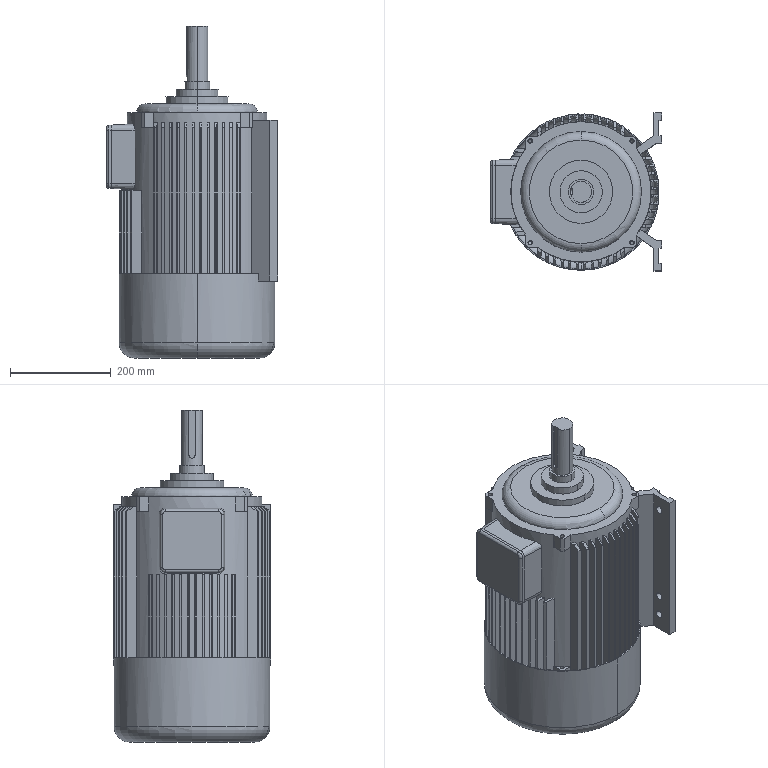Part | SolidWorks | features BaseBody 1 | 1 solid | 626 faces | box 340 x 314 x 660 mm | volume 8782416 mm3 | plane 303 | cylinder 171 | cone 140 | torus 12 | commonest cylinder face diameters 310 x50 6.8 x36 9 x16 10 x12 15 x12 279 x8